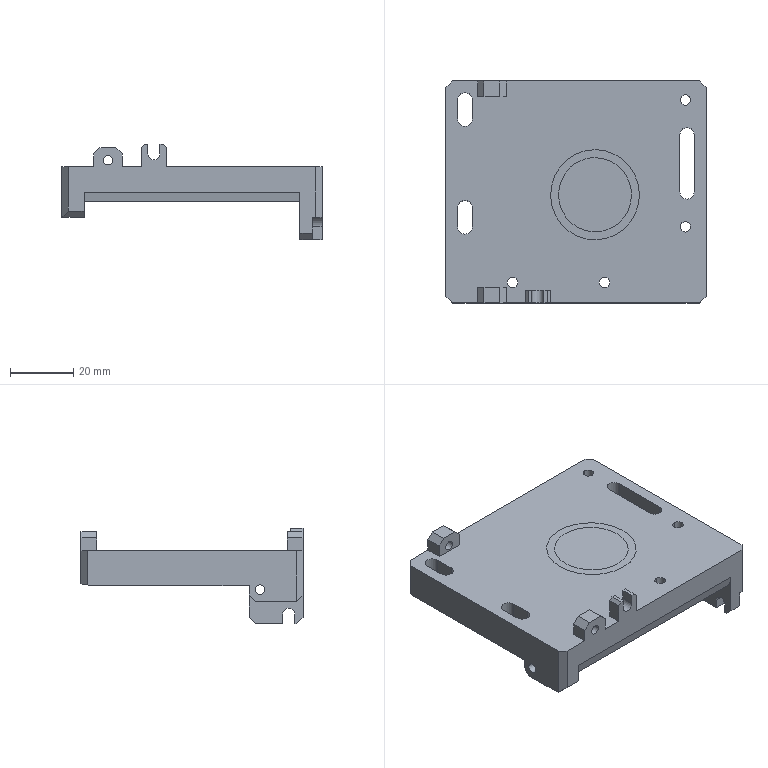NC program | NX | posted with a generic post | part box 82 x 70 x 30 mm
Lines 2119 to 3882 of 5501, first 1664 of 1756 lines:
(CAVITY_MILL_COPY_COPY_1 , TOOL : D4)
N4230 T04 M6
N4232 G54
N4234 G17 G0 G90 X-28.2 Y14.17 B0. C0. S9500 M3
N4236 G43 Z30. H4
N4238 Z1.25
N4240 G94 G1 Z-0.25 F1000.
N4242 X-28.364 Y14.123
N4244 G3 X-29.062 Y13.407 R1.
N4246 G2 X-30.376 Y12. R2. F1100.
N4248 X-29.062 Y10.593 R2.
N4250 G3 X-28.364 Y9.877 R1.
N4252 G1 X-28.2 Y9.83
N4254 Z1.25
N4256 G0 Y14.17 Z1.
N4258 G1 Z-0.5 F1000.
N4260 X-28.364 Y14.123
N4262 G3 X-29.062 Y13.407 R1.
N4264 G2 X-30.376 Y12. R2. F1100.
N4266 X-29.062 Y10.593 R2.
N4268 G3 X-28.364 Y9.877 R1.
N4270 G1 X-28.2 Y9.83
N4272 Z1.
N4274 G0 Y14.17 Z0.75
N4276 G1 Z-0.75 F1000.
N4278 X-28.364 Y14.123
N4280 G3 X-29.062 Y13.407 R1.
N4282 G2 X-30.376 Y12. R2. F1100.
N4284 X-29.062 Y10.593 R2.
N4286 G3 X-28.364 Y9.877 R1.
N4288 G1 X-28.2 Y9.83
N4290 Z0.75
N4292 G0 Y14.17 Z0.5
N4294 G1 Z-1. F1000.
N4296 X-28.364 Y14.123
N4298 G3 X-29.062 Y13.407 R1.
N4300 G2 X-30.376 Y12. R2. F1100.
N4302 X-29.062 Y10.593 R2.
N4304 G3 X-28.364 Y9.877 R1.
N4306 G1 X-28.2 Y9.83
N4308 Z0.5
N4310 G0 X-28.15 Y21.012 Z0.2
N4312 G1 Z-1.3 F1000.
N4314 X-29.294 Y20.491
N4316 G3 X-29.875 Y19.677 R1.
N4318 G1 X-31.666 Y19.85
N4320 X-31.661 Y19.9 F1100.
N4322 X-33.397
N4324 Y19.8
N4326 X-31.671
N4328 X-31.666 Y19.85
N4330 X-29.875 Y19.677
N4332 X-29.872 Y19.706
N4334 G2 X-28.845 Y21.476 R2.52
N4336 G1 X-28.779 Y21.523
N4338 G3 X-28.662 Y22.214 R0.5
N4340 G2 X-30. Y21.7 R2.
N4342 G1 X-35.
N4344 G2 X-36.492 Y22.373 R2.009
N4346 G3 X-36.51 Y21.738 R0.5
N4348 X-35.197 Y21.229 R2.489
N4350 G1 Y18.472
N4352 G3 X-36.491 Y17.982 R2.48
N4354 X-36.48 Y17.346 R0.5
N4356 G2 X-35. Y18. R2.
N4358 G1 X-31.
N4360 G2 X-29.368 Y17.156 R2.
N4362 G3 X-29.319 Y17.841 R0.5
N4364 G2 X-29.875 Y19.677 R2.52
N4366 X-29.294 Y20.491 R1.
N4368 G1 X-28.15 Y21.012
N4370 Z0.2
N4372 G0 X-28.445 Y17.989 Z-0.1
N4374 G1 Z-1.6 F1000.
N4376 X-29.322 Y18.673
N4378 G2 X-29.697 Y19.6 R1.
N4380 X-28.743 Y21.245 R2.52 F1100.
N4382 G3 X-28.642 Y21.931 R0.5
N4384 G2 X-30. Y21.4 R2.
N4386 G1 X-35.
N4388 G2 X-36.608 Y22.214 R2.003
N4390 G3 X-36.685 Y21.582 R0.5
N4392 X-35.197 Y20.928 R2.483
N4394 G1 Y18.472
N4396 G3 X-36.587 Y17.906 R2.48
N4398 X-36.544 Y17.271 R0.5
N4400 G2 X-35. Y18. R2.
N4402 G1 X-31.
N4404 G2 X-29.313 Y17.074 R2.
N4406 G3 X-29.23 Y17.756 R0.5
N4408 G2 X-29.697 Y19.6 R2.52
N4410 X-29.083 Y20.388 R1.
N4412 G1 X-28.053 Y20.806
N4414 Z-0.1
N4416 G0 X-28.354 Y17.868 Z-0.4
N4418 G1 Z-1.9 F1000.
N4420 X-29.2 Y18.616
N4422 G2 X-29.519 Y19.563 R1.
N4424 X-28.68 Y20.985 R2.52 F1100.
N4426 G3 X-28.604 Y21.667 R0.5
N4428 G2 X-30. Y21.1 R2.
N4430 G1 X-35.
N4432 G2 X-36.599 Y21.901 R2.004
N4434 G3 X-36.67 Y21.269 R0.5
N4436 X-35.197 Y20.628 R2.484
N4438 G1 Y18.472
N4440 G3 X-36.662 Y17.841 R2.48
N4442 X-36.594 Y17.208 R0.5
N4444 G2 X-35. Y18. R2.
N4446 G1 X-31.
N4448 G2 X-29.263 Y16.992 R2.
N4450 G3 X-29.147 Y17.668 R0.5
N4452 G2 X-29.519 Y19.563 R2.52
N4454 X-28.857 Y20.313 R1.
N4456 G1 X-27.937 Y20.622
N4458 Z-0.4
N4460 G0 X-28.263 Y17.735 Z-0.7
N4462 G1 Z-2.2 F1000.
N4464 X-29.073 Y18.546
N4466 G2 X-29.33 Y19.513 R1.
N4468 X-28.614 Y20.702 R2.52 F1100.
N4470 G1 X-28.516 Y20.793
N4472 G3 X-28.486 Y21.494 R0.5
N4474 G2 X-30. Y20.8 R2.
N4476 G1 X-35.
N4478 G2 X-36.681 Y21.717 R2.
N4480 G3 X-36.798 Y21.091 R0.5
N4482 X-35.197 Y20.328 R2.48
N4484 G1 Y18.472
N4486 G3 X-36.741 Y17.766 R2.48
N4488 X-36.645 Y17.137 R0.5
N4490 G2 X-35. Y18. R2.
N4492 G1 X-31.
N4494 G2 X-29.215 Y16.901 R2.
N4496 G3 X-29.064 Y17.571 R0.5
N4498 G2 X-29.33 Y19.513 R2.52
N4500 X-28.622 Y20.219 R1.
N4502 G1 X-27.77 Y20.446
N4504 Z-0.7
N4506 G0 X-28.192 Y17.619 Z-1.
N4508 G1 Z-2.5 F1000.
N4510 X-28.966 Y18.482
N4512 G2 X-29.172 Y19.461 R1.
N4514 X-28.537 Y20.481 R2.52 F1100.
N4516 G3 X-28.509 Y21.167 R0.5
N4518 G2 X-30. Y20.5 R2.
N4520 G1 X-35.
N4522 G2 X-36.694 Y21.437 R2.
N4524 G3 X-36.818 Y20.813 R0.5
N4526 X-35.197 Y20.028 R2.48
N4528 G1 Y18.472
N4530 G3 X-36.808 Y17.698 R2.48
N4532 X-36.688 Y17.073 R0.5
N4534 G2 X-35. Y18. R2.
N4536 G1 X-31.
N4538 G2 X-29.177 Y16.823 R2.
N4540 G3 X-28.998 Y17.486 R0.5
N4542 G2 X-29.172 Y19.461 R2.52
N4544 X-28.428 Y20.129 R1.
N4546 G1 X-27.713 Y20.279
N4548 Z-1.
N4550 G0 X-28.121 Y17.491 Z-1.3
N4552 G1 Z-2.8 F1000.
N4554 X-28.855 Y18.407
N4556 G2 X-29.006 Y19.396 R1.
N4558 X-28.466 Y20.235 R2.52 F1100.
N4560 G3 X-28.461 Y20.926 R0.5
N4562 G2 X-30. Y20.2 R2.004
N4564 G1 X-35.
N4566 G2 X-36.73 Y21.199 R2.003
N4568 G3 X-36.876 Y20.58 R0.5
N4570 X-35.197 Y19.728 R2.483
N4572 G1 Y18.472
N4574 G3 X-36.872 Y17.627 R2.48
N4576 X-36.728 Y17.007 R0.5
N4578 G2 X-35. Y18. R2.
N4580 G1 X-31.
N4582 G2 X-29.141 Y16.738 R2.
N4584 G3 X-28.931 Y17.392 R0.5
N4586 G2 X-29.006 Y19.396 R2.52
N4588 X-28.225 Y20.021 R1.
N4590 G1 X-27.613 Y20.114
N4592 Z-1.3
N4594 G0 X-28.078 Y17.405 Z-1.6
N4596 G1 Z-3.1 F1000.
N4598 X-28.783 Y18.356
N4600 G2 X-28.898 Y19.349 R1.
N4602 X-28.435 Y20.059 R2.52 F1100.
N4604 G3 X-28.443 Y20.745 R0.5
N4606 G2 X-30. Y20. R2.
N4608 G1 X-35.
N4610 G2 X-36.753 Y21.037 R2.
N4612 G3 X-36.912 Y20.421 R0.5
N4614 X-35.198 Y19.528 R2.48
N4616 G1 Y18.472
N4618 G3 X-36.912 Y17.579 R2.48
N4620 X-36.753 Y16.963 R0.5
N4622 G2 X-35. Y18. R2.
N4624 G1 X-31.
N4626 G2 X-29.12 Y16.682 R2.
N4628 G3 X-28.89 Y17.329 R0.5
N4630 G2 X-28.898 Y19.349 R2.52
N4632 X-28.095 Y19.945 R1.
N4634 G1 X-27.563 Y20.007
N4636 Z-1.6
N4638 G0 X-28.078 Y17.405 Z-1.9
N4640 G1 Z-3.4 F1000.
N4642 X-28.783 Y18.356
N4644 G2 X-28.898 Y19.349 R1.
N4646 X-28.435 Y20.059 R2.52 F1100.
N4648 G3 X-28.442 Y20.745 R0.5
N4650 G2 X-30. Y20. R2.
N4652 G1 X-35.
N4654 G2 X-36.753 Y21.037 R2.
N4656 G3 X-36.912 Y20.421 R0.5
N4658 X-35.198 Y19.528 R2.48
N4660 G1 Y18.472
N4662 G3 X-36.912 Y17.579 R2.48
N4664 X-36.753 Y16.963 R0.5
N4666 G2 X-35. Y18. R2.
N4668 G1 X-31.
N4670 G2 X-29.12 Y16.682 R2.
N4672 G3 X-28.89 Y17.329 R0.5
N4674 G2 X-28.898 Y19.349 R2.52
N4676 X-28.095 Y19.945 R1.
N4678 G1 X-27.563 Y20.007
N4680 Z-1.9
N4682 G0 X-28.078 Y17.405 Z-2.2
N4684 G1 Z-3.7 F1000.
N4686 X-28.783 Y18.356
N4688 G2 X-28.898 Y19.349 R1.
N4690 X-28.435 Y20.059 R2.52 F1100.
N4692 G3 X-28.442 Y20.745 R0.5
N4694 G2 X-30. Y20. R2.
N4696 G1 X-35.
N4698 G2 X-36.753 Y21.037 R2.
N4700 G3 X-36.912 Y20.421 R0.5
N4702 X-35.198 Y19.528 R2.48
N4704 G1 Y18.472
N4706 G3 X-36.912 Y17.579 R2.48
N4708 X-36.753 Y16.963 R0.5
N4710 G2 X-35. Y18. R2.
N4712 G1 X-31.
N4714 G2 X-29.12 Y16.682 R2.
N4716 G3 X-28.89 Y17.329 R0.5
N4718 G2 X-28.898 Y19.349 R2.52
N4720 X-28.095 Y19.945 R1.
N4722 G1 X-27.563 Y20.007
N4724 Z-2.2
N4726 G0 X-28.078 Y17.405 Z-2.5
N4728 G1 Z-4. F1000.
N4730 X-28.783 Y18.356
N4732 G2 X-28.898 Y19.349 R1.
N4734 X-28.435 Y20.059 R2.52 F1100.
N4736 G3 X-28.443 Y20.745 R0.5
N4738 G2 X-30. Y20. R2.
N4740 G1 X-35.
N4742 G2 X-36.753 Y21.037 R2.
N4744 G3 X-36.912 Y20.421 R0.5
N4746 X-35.198 Y19.528 R2.48
N4748 G1 Y18.472
N4750 G3 X-36.912 Y17.579 R2.48
N4752 X-36.753 Y16.963 R0.5
N4754 G2 X-35. Y18. R2.
N4756 G1 X-31.
N4758 G2 X-29.12 Y16.682 R2.
N4760 G3 X-28.89 Y17.329 R0.5
N4762 G2 X-28.898 Y19.349 R2.52
N4764 X-28.095 Y19.945 R1.
N4766 G1 X-27.563 Y20.007
N4768 Z-2.5
N4770 G0 X-28.078 Y17.405 Z-2.8
N4772 G1 Z-4.3 F1000.
N4774 X-28.783 Y18.356
N4776 G2 X-28.898 Y19.349 R1.
N4778 X-28.435 Y20.059 R2.52 F1100.
N4780 G3 X-28.443 Y20.745 R0.5
N4782 G2 X-30. Y20. R2.
N4784 G1 X-35.
N4786 G2 X-36.753 Y21.037 R2.
N4788 G3 X-36.912 Y20.421 R0.5
N4790 X-35.198 Y19.528 R2.48
N4792 G1 Y18.472
N4794 G3 X-36.912 Y17.579 R2.48
N4796 X-36.753 Y16.963 R0.5
N4798 G2 X-35. Y18. R2.
N4800 G1 X-31.
N4802 G2 X-29.12 Y16.682 R2.
N4804 G3 X-28.89 Y17.329 R0.5
N4806 G2 X-28.898 Y19.349 R2.52
N4808 X-28.095 Y19.945 R1.
N4810 G1 X-27.563 Y20.007
N4812 Z-2.8
N4814 G0 X-28.078 Y17.405 Z-3.1
N4816 G1 Z-4.6 F1000.
N4818 X-28.783 Y18.356
N4820 G2 X-28.898 Y19.349 R1.
N4822 X-28.435 Y20.059 R2.52 F1100.
N4824 G3 X-28.443 Y20.745 R0.5
N4826 G2 X-30. Y20. R2.
N4828 G1 X-35.
N4830 G2 X-36.753 Y21.037 R2.
N4832 G3 X-36.912 Y20.421 R0.5
N4834 X-35.198 Y19.528 R2.48
N4836 G1 Y18.472
N4838 G3 X-36.912 Y17.579 R2.48
N4840 X-36.753 Y16.963 R0.5
N4842 G2 X-35. Y18. R2.
N4844 G1 X-31.
N4846 G2 X-29.12 Y16.682 R2.
N4848 G3 X-28.89 Y17.329 R0.5
N4850 G2 X-28.898 Y19.349 R2.52
N4852 X-28.095 Y19.945 R1.
N4854 G1 X-27.563 Y20.007
N4856 Z-3.1
N4858 G0 X-28.078 Y17.405 Z-3.4
N4860 G1 Z-4.9 F1000.
N4862 X-28.783 Y18.356
N4864 G2 X-28.898 Y19.349 R1.
N4866 X-28.435 Y20.059 R2.52 F1100.
N4868 G3 X-28.443 Y20.745 R0.5
N4870 G2 X-30. Y20. R2.
N4872 G1 X-35.
N4874 G2 X-36.753 Y21.037 R2.
N4876 G3 X-36.912 Y20.421 R0.5
N4878 X-35.198 Y19.528 R2.48
N4880 G1 Y18.472
N4882 G3 X-36.912 Y17.579 R2.48
N4884 X-36.753 Y16.963 R0.5
N4886 G2 X-35. Y18. R2.
N4888 G1 X-31.
N4890 G2 X-29.12 Y16.682 R2.
N4892 G3 X-28.89 Y17.329 R0.5
N4894 G2 X-28.898 Y19.349 R2.52
N4896 X-28.095 Y19.945 R1.
N4898 G1 X-27.563 Y20.007
N4900 Z-3.4
N4902 G0 X-28.078 Y17.405 Z-3.7
N4904 G1 Z-5.2 F1000.
N4906 X-28.783 Y18.356
N4908 G2 X-28.898 Y19.349 R1.
N4910 X-28.435 Y20.059 R2.52 F1100.
N4912 G3 X-28.443 Y20.745 R0.5
N4914 G2 X-30. Y20. R2.
N4916 G1 X-35.
N4918 G2 X-36.753 Y21.037 R2.
N4920 G3 X-36.912 Y20.421 R0.5
N4922 X-35.198 Y19.528 R2.48
N4924 G1 Y18.472
N4926 G3 X-36.912 Y17.579 R2.48
N4928 X-36.753 Y16.963 R0.5
N4930 G2 X-35. Y18. R2.
N4932 G1 X-31.
N4934 G2 X-29.12 Y16.682 R2.
N4936 G3 X-28.89 Y17.329 R0.5
N4938 G2 X-28.898 Y19.349 R2.52
N4940 X-28.095 Y19.945 R1.
N4942 G1 X-27.563 Y20.007
N4944 Z-3.7
N4946 G0 X-28.078 Y17.405 Z-4.
N4948 G1 Z-5.5 F1000.
N4950 X-28.783 Y18.356
N4952 G2 X-28.898 Y19.349 R1.
N4954 X-28.435 Y20.059 R2.52 F1100.
N4956 G3 X-28.443 Y20.745 R0.5
N4958 G2 X-30. Y20. R2.
N4960 G1 X-35.
N4962 G2 X-36.753 Y21.037 R2.
N4964 G3 X-36.912 Y20.421 R0.5
N4966 X-35.198 Y19.528 R2.48
N4968 G1 Y18.472
N4970 G3 X-36.912 Y17.579 R2.48
N4972 X-36.753 Y16.963 R0.5
N4974 G2 X-35. Y18. R2.
N4976 G1 X-31.
N4978 G2 X-29.12 Y16.682 R2.
N4980 G3 X-28.89 Y17.329 R0.5
N4982 G2 X-28.898 Y19.349 R2.52
N4984 X-28.095 Y19.945 R1.
N4986 G1 X-27.563 Y20.007
N4988 Z-4.
N4990 G0 X-28.078 Y17.405 Z-4.3
N4992 G1 Z-5.8 F1000.
N4994 X-28.783 Y18.356
N4996 G2 X-28.898 Y19.349 R1.
N4998 X-28.435 Y20.059 R2.52 F1100.
N5000 G3 X-28.443 Y20.745 R0.5
N5002 G2 X-30. Y20. R2.
N5004 G1 X-35.
N5006 G2 X-36.753 Y21.037 R2.
N5008 G3 X-36.912 Y20.421 R0.5
N5010 X-35.198 Y19.528 R2.48
N5012 G1 Y18.472
N5014 G3 X-36.912 Y17.579 R2.48
N5016 X-36.753 Y16.963 R0.5
N5018 G2 X-35. Y18. R2.
N5020 G1 X-31.
N5022 G2 X-29.12 Y16.682 R2.
N5024 G3 X-28.89 Y17.329 R0.5
N5026 G2 X-28.898 Y19.349 R2.52
N5028 X-28.095 Y19.945 R1.
N5030 G1 X-27.563 Y20.007
N5032 Z-4.3
N5034 G0 X-28.078 Y17.405 Z-4.6
N5036 G1 Z-6.1 F1000.
N5038 X-28.783 Y18.356
N5040 G2 X-28.898 Y19.349 R1.
N5042 X-28.435 Y20.059 R2.52 F1100.
N5044 G3 X-28.443 Y20.745 R0.5
N5046 G2 X-30. Y20. R2.
N5048 G1 X-35.
N5050 G2 X-36.753 Y21.037 R2.
N5052 G3 X-36.912 Y20.421 R0.5
N5054 X-35.198 Y19.528 R2.48
N5056 G1 Y18.472
N5058 G3 X-36.912 Y17.579 R2.48
N5060 X-36.753 Y16.963 R0.5
N5062 G2 X-35. Y18. R2.
N5064 G1 X-31.
N5066 G2 X-29.12 Y16.682 R2.
N5068 G3 X-28.89 Y17.329 R0.5
N5070 G2 X-28.898 Y19.349 R2.52
N5072 X-28.095 Y19.945 R1.
N5074 G1 X-27.563 Y20.007
N5076 Z-4.6
N5078 G0 X-28.078 Y17.405 Z-4.9
N5080 G1 Z-6.4 F1000.
N5082 X-28.783 Y18.356
N5084 G2 X-28.898 Y19.349 R1.
N5086 X-28.435 Y20.059 R2.52 F1100.
N5088 G3 X-28.443 Y20.745 R0.5
N5090 G2 X-30. Y20. R2.
N5092 G1 X-35.
N5094 G2 X-36.753 Y21.037 R2.
N5096 G3 X-36.912 Y20.421 R0.5
N5098 X-35.198 Y19.528 R2.48
N5100 G1 Y18.472
N5102 G3 X-36.912 Y17.579 R2.48
N5104 X-36.753 Y16.963 R0.5
N5106 G2 X-35. Y18. R2.
N5108 G1 X-31.
N5110 G2 X-29.12 Y16.682 R2.
N5112 G3 X-28.89 Y17.329 R0.5
N5114 G2 X-28.898 Y19.349 R2.52
N5116 X-28.095 Y19.945 R1.
N5118 G1 X-27.563 Y20.007
N5120 Z-4.9
N5122 G0 X-28.078 Y17.405 Z-5.2
N5124 G1 Z-6.7 F1000.
N5126 X-28.783 Y18.356
N5128 G2 X-28.898 Y19.349 R1.
N5130 X-28.435 Y20.059 R2.52 F1100.
N5132 G3 X-28.443 Y20.745 R0.5
N5134 G2 X-30. Y20. R2.
N5136 G1 X-35.
N5138 G2 X-36.753 Y21.037 R2.
N5140 G3 X-36.912 Y20.421 R0.5
N5142 X-35.198 Y19.528 R2.48
N5144 G1 Y18.472
N5146 G3 X-36.912 Y17.579 R2.48
N5148 X-36.753 Y16.963 R0.5
N5150 G2 X-35. Y18. R2.
N5152 G1 X-31.
N5154 G2 X-29.12 Y16.682 R2.
N5156 G3 X-28.89 Y17.329 R0.5
N5158 G2 X-28.898 Y19.349 R2.52
N5160 X-28.095 Y19.945 R1.
N5162 G1 X-27.563 Y20.007
N5164 Z-5.2
N5166 G0 X-28.078 Y17.405 Z-5.5
N5168 G1 Z-7. F1000.
N5170 X-28.783 Y18.356
N5172 G2 X-28.898 Y19.349 R1.
N5174 X-28.435 Y20.059 R2.52 F1100.
N5176 G3 X-28.443 Y20.745 R0.5
N5178 G2 X-30. Y20. R2.
N5180 G1 X-35.
N5182 G2 X-36.753 Y21.037 R2.
N5184 G3 X-36.912 Y20.421 R0.5
N5186 X-35.198 Y19.528 R2.48
N5188 G1 Y18.472
N5190 G3 X-36.912 Y17.579 R2.48
N5192 X-36.753 Y16.963 R0.5
N5194 G2 X-35. Y18. R2.
N5196 G1 X-31.
N5198 G2 X-29.12 Y16.682 R2.
N5200 G3 X-28.89 Y17.329 R0.5
N5202 G2 X-28.898 Y19.349 R2.52
N5204 X-28.095 Y19.945 R1.
N5206 G1 X-27.563 Y20.007
N5208 Z-5.5
N5210 G0 Z30.
N5212 X-28.2 Y14.17
N5214 Z0.2
N5216 G1 Z-1.3 F1000.
N5218 X-28.364 Y14.123
N5220 G3 X-29.062 Y13.407 R1.
N5222 G2 X-30.376 Y12. R2. F1100.
N5224 X-29.062 Y10.593 R2.
N5226 G3 X-28.364 Y9.877 R1.
N5228 G1 X-28.2 Y9.83
N5230 Z0.2
N5232 G0 Y14.17 Z-0.1
N5234 G1 Z-1.6 F1000.
N5236 X-28.364 Y14.123
N5238 G3 X-29.062 Y13.407 R1.
N5240 G2 X-30.376 Y12. R2. F1100.
N5242 X-29.062 Y10.593 R2.
N5244 G3 X-28.364 Y9.877 R1.
N5246 G1 X-28.2 Y9.83
N5248 Z-0.1
N5250 G0 Y14.17 Z-0.4
N5252 G1 Z-1.9 F1000.
N5254 X-28.364 Y14.123
N5256 G3 X-29.062 Y13.407 R1.
N5258 G2 X-30.376 Y12. R2. F1100.
N5260 X-29.062 Y10.593 R2.
N5262 G3 X-28.364 Y9.877 R1.
N5264 G1 X-28.2 Y9.83
N5266 Z-0.4
N5268 G0 Y14.17 Z-0.7
N5270 G1 Z-2.2 F1000.
N5272 X-28.364 Y14.123
N5274 G3 X-29.062 Y13.407 R1.
N5276 G2 X-30.376 Y12. R2. F1100.
N5278 X-29.062 Y10.593 R2.
N5280 G3 X-28.364 Y9.877 R1.
N5282 G1 X-28.2 Y9.83
N5284 Z-0.7
N5286 G0 Y14.17 Z-1.
N5288 G1 Z-2.5 F1000.
N5290 X-28.364 Y14.123
N5292 G3 X-29.062 Y13.407 R1.
N5294 G2 X-30.376 Y12. R2. F1100.
N5296 X-29.062 Y10.593 R2.
N5298 G3 X-28.364 Y9.877 R1.
N5300 G1 X-28.2 Y9.83
N5302 Z-1.
N5304 G0 Y14.17 Z-1.3
N5306 G1 Z-2.8 F1000.
N5308 X-28.364 Y14.123
N5310 G3 X-29.062 Y13.407 R1.
N5312 G2 X-30.376 Y12. R2. F1100.
N5314 X-29.062 Y10.593 R2.
N5316 G3 X-28.364 Y9.877 R1.
N5318 G1 X-28.2 Y9.83
N5320 Z-1.3
N5322 G0 Y14.17 Z-1.6
N5324 G1 Z-3.1 F1000.
N5326 X-28.364 Y14.123
N5328 G3 X-29.062 Y13.407 R1.
N5330 G2 X-29.372 Y12.738 R2. F1100.
N5332 X-30.355 Y12. R1.958
N5334 X-29.375 Y11.265 R1.952
N5336 X-29.062 Y10.593 R2.
N5338 G3 X-28.364 Y9.877 R1.
N5340 G1 X-28.2 Y9.83
N5342 Z-1.6
N5344 G0 Y14.156 Z-1.9
N5346 G1 Z-3.4 F1000.
N5348 X-28.366 Y14.107
N5350 G3 X-29.053 Y13.381 R1.
N5352 G2 X-30.252 Y12. R1.977 F1100.
N5354 X-29.052 Y10.612 R1.979
N5356 G3 X-28.367 Y9.884 R1.
N5358 G1 X-28.2 Y9.833
N5360 Z-1.9
N5362 G0 Y14.124 Z-2.2
N5364 G1 Z-3.7 F1000.
N5366 X-28.373 Y14.069
N5368 G3 X-29.045 Y13.329 R1.
N5370 G2 X-30.05 Y12.001 R1.981 F1100.
N5372 X-29.049 Y10.685 R1.988
N5374 G3 X-28.37 Y9.95 R1.
N5376 G1 X-28.2 Y9.897
N5378 Z-2.2
N5380 G0 Y14.094 Z-2.5
N5382 G1 Z-4. F1000.
N5384 X-28.388 Y14.025
N5386 G3 X-29.031 Y13.26 R1.
N5388 G2 X-29.805 Y11.996 R2.023 F1100.
N5390 X-29.034 Y10.765 R1.987
N5392 G3 X-28.383 Y10.006 R1.
N5394 G1 X-28.2 Y9.941
N5396 Z-2.5
N5398 G0 Y13.998 Z-2.8
N5400 G1 Z-4.3 F1000.
N5402 X-28.409 Y13.911
N5404 G3 X-29.016 Y13.116 R1.
N5406 G2 X-29.552 Y12.002 R1.969 F1100.
N5408 X-29.018 Y10.89 R1.99
N5410 G3 X-28.407 Y10.098 R1.
N5412 G1 X-28.2 Y10.012
N5414 Z-2.8
N5416 G0 Y13.908 Z-3.1
N5418 G1 Z-4.6 F1000.
N5420 X-28.462 Y13.772
N5422 G3 X-29.002 Y12.93 R1.
N5424 G2 X-29.272 Y12.002 R2.068 F1100.
N5426 X-29.001 Y11.043 R2.095
N5428 G3 X-28.471 Y10.195 R1.
N5430 G1 X-28.2 Y10.051
N5432 Z-3.1
N5434 G0 Z30.
N5436 X-37.8 Y9.83
N5438 Z1.25
N5440 G1 Z-0.25 F1000.
N5442 X-37.636 Y9.877
N5444 G3 X-36.938 Y10.593 R1.
N5446 G2 X-35.625 Y12. R2. F1100.
N5448 X-36.938 Y13.407 R2.
N5450 G3 X-37.636 Y14.123 R1.
N5452 G1 X-37.8 Y14.17
N5454 Z1.25
N5456 G0 Y9.83 Z1.
N5458 G1 Z-0.5 F1000.
N5460 X-37.636 Y9.877
N5462 G3 X-36.938 Y10.593 R1.
N5464 G2 X-35.625 Y12. R2. F1100.
N5466 X-36.938 Y13.407 R2.
N5468 G3 X-37.636 Y14.123 R1.
N5470 G1 X-37.8 Y14.17
N5472 Z1.
N5474 G0 Y9.83 Z0.75
N5476 G1 Z-0.75 F1000.
N5478 X-37.636 Y9.877
N5480 G3 X-36.938 Y10.593 R1.
N5482 G2 X-35.625 Y12. R2. F1100.
N5484 X-36.938 Y13.407 R2.
N5486 G3 X-37.636 Y14.123 R1.
N5488 G1 X-37.8 Y14.17
N5490 Z0.75
N5492 G0 Y9.83 Z0.5
N5494 G1 Z-1. F1000.
N5496 X-37.636 Y9.877
N5498 G3 X-36.938 Y10.593 R1.
N5500 G2 X-35.625 Y12. R2. F1100.
N5502 X-36.938 Y13.407 R2.
N5504 G3 X-37.636 Y14.123 R1.
N5506 G1 X-37.8 Y14.17
N5508 Z0.5
N5510 G0 Y9.83 Z0.2
N5512 G1 Z-1.3 F1000.
N5514 X-37.636 Y9.877
N5516 G3 X-36.938 Y10.593 R1.
N5518 G2 X-35.625 Y12. R2. F1100.
N5520 X-36.938 Y13.407 R2.
N5522 G3 X-37.636 Y14.123 R1.
N5524 G1 X-37.8 Y14.17
N5526 Z0.2
N5528 G0 Y9.83 Z-0.1
N5530 G1 Z-1.6 F1000.
N5532 X-37.636 Y9.877
N5534 G3 X-36.938 Y10.593 R1.
N5536 G2 X-35.625 Y12. R2. F1100.
N5538 X-36.938 Y13.407 R2.
N5540 G3 X-37.636 Y14.123 R1.
N5542 G1 X-37.8 Y14.17
N5544 Z-0.1
N5546 G0 Y9.83 Z-0.4
N5548 G1 Z-1.9 F1000.
N5550 X-37.636 Y9.877
N5552 G3 X-36.938 Y10.593 R1.
N5554 G2 X-35.625 Y12. R2. F1100.
N5556 X-36.938 Y13.407 R2.
N5558 G3 X-37.636 Y14.123 R1.
N5560 G1 X-37.8 Y14.17
N5562 Z-0.4
N5564 G0 Y9.83 Z-0.7
N5566 G1 Z-2.2 F1000.
N5568 X-37.636 Y9.877
N5570 G3 X-36.938 Y10.593 R1.
N5572 G2 X-35.625 Y12. R2. F1100.
N5574 X-36.938 Y13.407 R2.
N5576 G3 X-37.636 Y14.123 R1.
N5578 G1 X-37.8 Y14.17
N5580 Z-0.7
N5582 G0 Y9.83 Z-1.
N5584 G1 Z-2.5 F1000.
N5586 X-37.636 Y9.877
N5588 G3 X-36.938 Y10.593 R1.
N5590 G2 X-35.625 Y12. R2. F1100.
N5592 X-36.938 Y13.407 R2.
N5594 G3 X-37.636 Y14.123 R1.
N5596 G1 X-37.8 Y14.17
N5598 Z-1.
N5600 G0 Y9.83 Z-1.3
N5602 G1 Z-2.8 F1000.
N5604 X-37.636 Y9.877
N5606 G3 X-36.938 Y10.593 R1.
N5608 G2 X-35.625 Y12. R2. F1100.
N5610 X-36.938 Y13.407 R2.
N5612 G3 X-37.636 Y14.123 R1.
N5614 G1 X-37.8 Y14.17
N5616 Z-1.3
N5618 G0 Y9.83 Z-1.6
N5620 G1 Z-3.1 F1000.
N5622 X-37.636 Y9.877
N5624 G3 X-36.938 Y10.593 R1.
N5626 G2 X-36.62 Y11.273 R2. F1100.
N5628 X-35.641 Y12. R1.936
N5630 X-36.715 Y12.871 R1.953
N5632 X-36.938 Y13.407 R2.
N5634 G3 X-37.636 Y14.123 R1.
N5636 G1 X-37.8 Y14.17
N5638 Z-1.6
N5640 G0 Y9.822 Z-1.9
N5642 G1 Z-3.4 F1000.
N5644 X-37.632 Y9.874
N5646 G3 X-36.95 Y10.605 R1.
N5648 G2 X-35.757 Y11.997 R1.981 F1100.
N5650 X-36.153 Y12.219 R3.507
N5652 X-36.604 Y12.647 R2.331
N5654 X-36.774 Y12.922 R2.63
N5656 X-36.953 Y13.401 R1.909
N5658 G3 X-37.632 Y14.135 R1.
N5660 G1 X-37.8 Y14.187
N5662 Z-1.9
N5664 G0 Y9.871 Z-2.2
N5666 G1 Z-3.7 F1000.
N5668 X-37.627 Y9.926
N5670 G3 X-36.954 Y10.666 R1.
N5672 G2 X-36.153 Y11.876 R2.005 F1100.
N5674 G1 X-35.994 Y11.984
N5676 X-35.959 Y11.997
N5678 G2 X-36.894 Y13.112 R2.069
N5680 X-36.954 Y13.324 R1.922
N5682 G3 X-37.63 Y14.061 R1.
N5684 G1 X-37.8 Y14.114
N5686 Z-2.2
N5688 G0 Y9.931 Z-2.5
N5690 G1 Z-4. F1000.
N5692 X-37.616 Y9.996
N5694 G3 X-36.967 Y10.757 R1.
N5696 G2 X-36.196 Y11.998 R2.003 F1100.
N5698 X-36.964 Y13.235 R2.022
N5700 G3 X-37.617 Y13.993 R1.
N5702 G1 X-37.8 Y14.056
N5704 Z-2.5
N5706 G0 Y10.025 Z-2.8
N5708 G1 Z-4.3 F1000.
N5710 X-37.595 Y10.108
N5712 G3 X-36.981 Y10.896 R1.
N5714 G2 X-36.452 Y11.998 R2.008 F1100.
N5716 X-36.98 Y13.099 R2.023
N5718 G3 X-37.596 Y13.887 R1.
N5720 G1 X-37.8 Y13.969
N5722 Z-2.8
N5724 G0 Y10.11 Z-3.1
N5726 G1 Z-4.6 F1000.
N5728 X-37.544 Y10.24
N5730 G3 X-36.997 Y11.078 R1.
N5732 G2 X-36.729 Y11.984 R2.046 F1100.
N5734 X-36.998 Y12.946 R2.256
N5736 G3 X-37.54 Y13.786 R1.
N5738 G1 X-37.8 Y13.919
N5740 Z-3.1
N5742 G0 Z30.
(FLOOR_WALL_1_COPY , TOOL : D4)
N5744 X38.187 Y31.917
N5746 Z0.5
N5748 G1 Z-1. F1250.
N5750 X37.2 Y31.346
N5752 G3 X37. Y31. R0.4
N5754 G1 Y22.
N5756 X35.2
N5758 Y31.
N5760 X33.4
N5762 Y22.
N5764 X31.6
N5766 Y31.
N5768 G2 X31.8 Y31.346 R0.4
N5770 G1 X33.798 Y32.5
N5772 Z0.5
N5774 G0 Z30.
N5776 X38.187 Y40.745
N5778 Z-5.5
N5780 G1 Z-7.
N5782 X37.2 Y40.175
N5784 G3 X37. Y39.828 R0.4
N5786 G1 Y33.2
N5788 X35.044
N5790 Y41.784
N5792 X33.828 Y43.
N5794 X33.089
N5796 Y33.2
N5798 X31.133
N5800 Y43.
N5802 X29.178
N5804 Y33.2
N5806 G3 X29.524 Y33.4 R0.4
N5808 G1 Z-5.5
N5810 G0 Z30.
N5812 X38.5 Y19.454
N5814 Z-5.5
N5816 G1 Z-7.
N5818 X36.8
N5820 G3 X37. Y19.8 R0.4
N5822 G1 Y-39.828
N5824 X35.044 Y-41.784
N5826 Y19.8
N5828 X33.089
N5830 Y-43.
N5832 X31.133
N5834 Y19.8
N5836 X29.178
N5838 Y-43.
N5840 X27.222
N5842 Y43.
N5844 X25.267
N5846 Y-43.
N5848 X23.311
N5850 Y43.
N5852 X21.356
N5854 Y-43.
N5856 X19.4
N5858 Y43.
N5860 X17.444
N5862 Y-43.
N5864 X15.489
N5866 Y43.
N5868 X13.533
N5870 Y-43.
N5872 X11.578
N5874 Y43.
N5876 X9.622
N5878 Y-43.
N5880 X7.667
N5882 Y43.
N5884 X5.711
N5886 Y-43.
N5888 X3.756
N5890 Y43.
N5892 X1.8
N5894 Y-43.
N5896 X-0.156
N5898 Y43.
N5900 X-2.111
N5902 Y-43.
N5904 X-4.067
N5906 Y43.
N5908 X-6.022
N5910 Y-43.
N5912 X-7.978
N5914 Y43.
N5916 X-9.933
N5918 Y-43.
N5920 X-11.889
N5922 Y43.
N5924 X-13.844
N5926 Y-43.
N5928 X-15.8
N5930 Y43.
N5932 X-17.756
N5934 Y-43.
N5936 X-19.711
N5938 Y43.
N5940 X-21.667
N5942 Y-43.
N5944 X-23.622
N5946 Y43.
N5948 X-25.578
N5950 Y-43.
N5952 X-27.533
N5954 Y43.
N5956 X-29.489
N5958 Y33.2
N5960 X-31.444
N5962 Y43.
N5964 X-33.4
N5966 Y33.2
N5968 X-35.356
N5970 Y41.473
N5972 G2 X-35.156 Y41.819 R0.4
N5974 G1 X-36.143 Y42.807
N5976 Z-5.5
N5978 G0 Z3.1
N5980 G1 X-29.489 Y33.2 F8000.
N5982 G0 Z-5.5
N5984 G1 Z-7. F1250.
N5986 X-28.
N5988 G2 X-27.8 Y33. R0.2
N5990 G1 Y20.
N5992 G2 X-28. Y19.8 R0.2
N5994 G1 X-29.489
N5996 Y18.2
N5998 X-31.444
N6000 Y19.8
N6002 X-33.4
N6004 Y18.2
N6006 X-35.356
N6008 Y19.8
N6010 Z-5.5
N6012 G0 Z3.1
N6014 G1 X-29.489 Y18.2 F8000.
N6016 G0 Z-5.5
N6018 G1 Z-7. F1250.
N6020 X-29.
N6022 G2 X-28.8 Y18. R0.2
N6024 G1 Y5.99
N6026 G2 X-29. Y5.8 R0.2
N6028 G1 X-29.489
N6030 Y-43.
N6032 X-31.444
N6034 Y5.8
N6036 X-33.4
N6038 Y-43.
N6040 X-33.828
N6042 X-35.356 Y-41.473
N6044 Y5.8
N6046 Z-5.5
N6048 G0 Z30.
N6050 X-38.5 Y20.198
N6052 Z-5.5
N6054 G1 Z-7.
N6056 X-37.346 Y18.2
N6058 G3 X-37. Y18. R0.4
N6060 G1 X-29.
N6062 Y6.
N6064 X-37.
N6066 G3 X-37.346 Y5.8 R0.4
N6068 G1 X-38.5 Y3.802
N6070 Z-5.5
N6072 G0 Z3.1
N6074 G1 X38.5 Y17.802 F8000.
N6076 G0 Z-5.5
N6078 G1 Z-7. F1250.
N6080 X37.346 Y19.8
N6082 G3 X37. Y20. R0.4
N6084 G1 X28.
N6086 Y33.
N6088 X37.
N6090 G3 X37.346 Y33.2 R0.4
N6092 G1 X38.5 Y35.198
N6094 Z-5.5
N6096 G0 Z3.1
N6098 G1 X-38.5 F8000.
N6100 G0 Z-5.5
N6102 G1 Z-7. F1250.
N6104 X-37.346 Y33.2
N6106 G3 X-37. Y33. R0.4
N6108 G1 X-28.
N6110 Y20.
N6112 X-37.
N6114 G3 X-37.346 Y19.8 R0.4
N6116 G1 X-38.5 Y17.802
N6118 Z-5.5
N6120 G0 Z30.
N6122 X-26.813 Y31.917
N6124 Z0.5
N6126 G1 Z-1.
N6128 X-27.8 Y31.346
N6130 G3 X-28. Y31. R0.4
N6132 G1 Y22.
N6134 X-29.8
N6136 Y31.
N6138 X-31.6
N6140 Y22.
N6142 X-33.4
N6144 Y31.
N6146 G2 X-33.2 Y31.346 R0.4
N6148 G1 X-31.202 Y32.5
N6150 Z0.5
N6152 G0 Z30.
N6154 M5
(CAVITY_MILL_COPY_COPY_2 , TOOL : D3)
N6156 T03 M6
N6158 G54
N6160 G17 G0 G90 X-36.448 Y12.379 B0. C0. S9500 M3
N6162 G43 Z30. H3
N6164 Z1.3
N6166 G94 G1 Z-0.2 F1000.
N6168 X-36.043 Y12.685
N6170 G2 X-35.826 Y11.709 R1.
N6172 G3 X-35.809 Y11.363 R0.5 F1100.
N6174 G2 X-35. Y11.6 R1.5
N6176 G1 X-31.
N6178 G2 X-30.191 Y11.363 R1.5
N6180 G3 X-30.386 Y11.983 R0.5
N6182 G1 X-30.404 Y11.99
N6184 Y12.01
N6186 X-30.386 Y12.017
N6188 G3 X-30.191 Y12.637 R0.5
N6190 G2 X-31. Y12.4 R1.5
N6192 G1 X-35.
N6194 G2 X-35.809 Y12.637 R1.5
N6196 G3 X-35.614 Y12.017 R0.5
N6198 G1 X-35.596 Y12.01
N6200 Y11.99
N6202 X-35.614 Y11.983
N6204 G3 X-35.826 Y11.709 R0.5
N6206 G2 X-36.563 Y11.033 R1.
N6208 G1 X-36.918 Y10.955
N6210 Z1.3
N6212 G0 X-36.448 Y12.379 Z1.1
N6214 G1 Z-0.4 F1000.
N6216 X-36.043 Y12.685
N6218 G2 X-35.826 Y11.709 R1.
N6220 G3 X-35.809 Y11.363 R0.5 F1100.
N6222 G2 X-35. Y11.6 R1.5
N6224 G1 X-31.
N6226 G2 X-30.191 Y11.363 R1.5
N6228 G3 X-30.386 Y11.983 R0.5
N6230 G1 X-30.404 Y11.99
N6232 Y12.01
N6234 X-30.386 Y12.017
N6236 G3 X-30.191 Y12.637 R0.5
N6238 G2 X-31. Y12.4 R1.5
N6240 G1 X-35.
N6242 G2 X-35.809 Y12.637 R1.5
N6244 G3 X-35.614 Y12.017 R0.5
N6246 G1 X-35.596 Y12.01
N6248 Y11.99
N6250 X-35.614 Y11.983
N6252 G3 X-35.826 Y11.709 R0.5
N6254 G2 X-36.563 Y11.033 R1.
N6256 G1 X-36.918 Y10.955
N6258 Z1.1
N6260 G0 X-36.448 Y12.379 Z0.9
N6262 G1 Z-0.6 F1000.
N6264 X-36.043 Y12.685
N6266 G2 X-35.826 Y11.709 R1.
N6268 G3 X-35.809 Y11.363 R0.5 F1100.
N6270 G2 X-35. Y11.6 R1.5
N6272 G1 X-31.
N6274 G2 X-30.191 Y11.363 R1.5
N6276 G3 X-30.386 Y11.983 R0.5
N6278 G1 X-30.404 Y11.99
N6280 Y12.01
N6282 X-30.386 Y12.017
N6284 G3 X-30.191 Y12.637 R0.5
N6286 G2 X-31. Y12.4 R1.5
N6288 G1 X-35.
N6290 G2 X-35.809 Y12.637 R1.5
N6292 G3 X-35.614 Y12.017 R0.5
N6294 G1 X-35.596 Y12.01
N6296 Y11.99
N6298 X-35.614 Y11.983
N6300 G3 X-35.826 Y11.709 R0.5
N6302 G2 X-36.563 Y11.033 R1.
N6304 G1 X-36.918 Y10.955
N6306 Z0.9
N6308 G0 X-36.448 Y12.379 Z0.7
N6310 G1 Z-0.8 F1000.
N6312 X-36.043 Y12.685
N6314 G2 X-35.826 Y11.709 R1.
N6316 G3 X-35.809 Y11.363 R0.5 F1100.
N6318 G2 X-35. Y11.6 R1.5
N6320 G1 X-31.
N6322 G2 X-30.191 Y11.363 R1.5
N6324 G3 X-30.386 Y11.983 R0.5
N6326 G1 X-30.404 Y11.99
N6328 Y12.01
N6330 X-30.386 Y12.017
N6332 G3 X-30.191 Y12.637 R0.5
N6334 G2 X-31. Y12.4 R1.5
N6336 G1 X-35.
N6338 G2 X-35.809 Y12.637 R1.5
N6340 G3 X-35.614 Y12.017 R0.5
N6342 G1 X-35.596 Y12.01
N6344 Y11.99
N6346 X-35.614 Y11.983
N6348 G3 X-35.826 Y11.709 R0.5
N6350 G2 X-36.563 Y11.033 R1.
N6352 G1 X-36.918 Y10.955
N6354 Z0.7
N6356 G0 X-36.448 Y12.379 Z0.5
N6358 G1 Z-1. F1000.
N6360 X-36.043 Y12.685
N6362 G2 X-35.826 Y11.709 R1.
N6364 G3 X-35.809 Y11.363 R0.5 F1100.
N6366 G2 X-35. Y11.6 R1.5
N6368 G1 X-31.
N6370 G2 X-30.191 Y11.363 R1.5
N6372 G3 X-30.386 Y11.983 R0.5
N6374 G1 X-30.404 Y11.99
N6376 Y12.01
N6378 X-30.386 Y12.017
N6380 G3 X-30.191 Y12.637 R0.5
N6382 G2 X-31. Y12.4 R1.5
N6384 G1 X-35.
N6386 G2 X-35.809 Y12.637 R1.5
N6388 G3 X-35.614 Y12.017 R0.5
N6390 G1 X-35.596 Y12.01
N6392 Y11.99
N6394 X-35.614 Y11.983
N6396 G3 X-35.826 Y11.709 R0.5
N6398 G2 X-36.563 Y11.033 R1.
N6400 G1 X-36.918 Y10.955
N6402 Z0.5
N6404 G0 X-36.448 Y12.379 Z0.3
N6406 G1 Z-1.2 F1000.
N6408 X-36.043 Y12.685
N6410 G2 X-35.826 Y11.709 R1.
N6412 G3 X-35.809 Y11.363 R0.5 F1100.
N6414 G2 X-35. Y11.6 R1.5
N6416 G1 X-31.
N6418 G2 X-30.191 Y11.363 R1.5
N6420 G3 X-30.386 Y11.983 R0.5
N6422 G1 X-30.404 Y11.99
N6424 Y12.01
N6426 X-30.386 Y12.017
N6428 G3 X-30.191 Y12.637 R0.5
N6430 G2 X-31. Y12.4 R1.5
N6432 G1 X-35.
N6434 G2 X-35.809 Y12.637 R1.5
N6436 G3 X-35.614 Y12.017 R0.5
N6438 G1 X-35.596 Y12.01
N6440 Y11.99
N6442 X-35.614 Y11.983
N6444 G3 X-35.826 Y11.709 R0.5
N6446 G2 X-36.563 Y11.033 R1.
N6448 G1 X-36.918 Y10.955
N6450 Z0.3
N6452 G0 X-36.448 Y12.379 Z0.1
N6454 G1 Z-1.4 F1000.
N6456 X-36.043 Y12.685
N6458 G2 X-35.826 Y11.709 R1.
N6460 G3 X-35.809 Y11.363 R0.5 F1100.
N6462 G2 X-35. Y11.6 R1.5
N6464 G1 X-31.
N6466 G2 X-30.191 Y11.363 R1.5
N6468 G3 X-30.386 Y11.983 R0.5
N6470 G1 X-30.404 Y11.99
N6472 Y12.01
N6474 X-30.386 Y12.017
N6476 G3 X-30.191 Y12.637 R0.5
N6478 G2 X-31. Y12.4 R1.5
N6480 G1 X-35.
N6482 G2 X-35.809 Y12.637 R1.5
N6484 G3 X-35.614 Y12.017 R0.5
N6486 G1 X-35.596 Y12.01
N6488 Y11.99
N6490 X-35.614 Y11.983
N6492 G3 X-35.826 Y11.709 R0.5
N6494 G2 X-36.563 Y11.033 R1.
N6496 G1 X-36.918 Y10.955
N6498 Z0.1
N6500 G0 X-36.448 Y12.379 Z-0.1
N6502 G1 Z-1.6 F1000.
N6504 X-36.043 Y12.685
N6506 G2 X-35.826 Y11.709 R1.
N6508 G3 X-35.809 Y11.363 R0.5 F1100.
N6510 G2 X-35. Y11.6 R1.5
N6512 G1 X-31.
N6514 G2 X-30.191 Y11.363 R1.5
N6516 G3 X-30.386 Y11.983 R0.5
N6518 G1 X-30.404 Y11.99
N6520 Y12.01
N6522 X-30.386 Y12.017
N6524 G3 X-30.191 Y12.637 R0.5
N6526 G2 X-31. Y12.4 R1.5
N6528 G1 X-35.
N6530 G2 X-35.809 Y12.637 R1.5
N6532 G3 X-35.614 Y12.017 R0.5
N6534 G1 X-35.596 Y12.01
N6536 Y11.99
N6538 X-35.614 Y11.983
N6540 G3 X-35.826 Y11.709 R0.5
N6542 G2 X-36.563 Y11.033 R1.
N6544 G1 X-36.918 Y10.955
N6546 Z-0.1
N6548 G0 X-36.448 Y12.379 Z-0.3
N6550 G1 Z-1.8 F1000.
N6552 X-36.043 Y12.685
N6554 G2 X-35.826 Y11.709 R1.
N6556 G3 X-35.809 Y11.363 R0.5 F1100.
N6558 G2 X-35. Y11.6 R1.5
N6560 G1 X-31.
N6562 G2 X-30.191 Y11.363 R1.5
N6564 G3 X-30.386 Y11.983 R0.5
N6566 G1 X-30.404 Y11.99
N6568 Y12.01
N6570 X-30.386 Y12.017
N6572 G3 X-30.191 Y12.637 R0.5
N6574 G2 X-31. Y12.4 R1.5
N6576 G1 X-35.
N6578 G2 X-35.809 Y12.637 R1.5
N6580 G3 X-35.614 Y12.017 R0.5
N6582 G1 X-35.596 Y12.01
N6584 Y11.99
N6586 X-35.614 Y11.983
N6588 G3 X-35.826 Y11.709 R0.5
N6590 G2 X-36.563 Y11.033 R1.
N6592 G1 X-36.918 Y10.955
N6594 Z-0.3
N6596 G0 X-36.448 Y12.379 Z-0.5
N6598 G1 Z-2. F1000.
N6600 X-36.043 Y12.685
N6602 G2 X-35.826 Y11.709 R1.
N6604 G3 X-35.809 Y11.363 R0.5 F1100.
N6606 G2 X-35. Y11.6 R1.5
N6608 G1 X-31.
N6610 G2 X-30.191 Y11.363 R1.5
N6612 G3 X-30.386 Y11.983 R0.5
N6614 G1 X-30.404 Y11.99
N6616 Y12.01
N6618 X-30.386 Y12.017
N6620 G3 X-30.191 Y12.637 R0.5
N6622 G2 X-31. Y12.4 R1.5
N6624 G1 X-35.
N6626 G2 X-35.809 Y12.637 R1.5
N6628 G3 X-35.614 Y12.017 R0.5
N6630 G1 X-35.596 Y12.01
N6632 Y11.99
N6634 X-35.614 Y11.983
N6636 G3 X-35.826 Y11.709 R0.5
N6638 G2 X-36.563 Y11.033 R1.
N6640 G1 X-36.918 Y10.955
N6642 Z-0.5
N6644 G0 X-36.448 Y12.379 Z-0.7
N6646 G1 Z-2.2 F1000.
N6648 X-36.043 Y12.685
N6650 G2 X-35.826 Y11.709 R1.
N6652 G3 X-35.809 Y11.363 R0.5 F1100.
N6654 G2 X-35. Y11.6 R1.5
N6656 G1 X-31.
N6658 G2 X-30.191 Y11.363 R1.5
N6660 G3 X-30.386 Y11.983 R0.5
N6662 G1 X-30.404 Y11.99
N6664 Y12.01
N6666 X-30.386 Y12.017
N6668 G3 X-30.191 Y12.637 R0.5
N6670 G2 X-31. Y12.4 R1.5
N6672 G1 X-35.
N6674 G2 X-35.809 Y12.637 R1.5
N6676 G3 X-35.614 Y12.017 R0.5
N6678 G1 X-35.596 Y12.01
N6680 Y11.99
N6682 X-35.614 Y11.983
N6684 G3 X-35.826 Y11.709 R0.5
N6686 G2 X-36.563 Y11.033 R1.
N6688 G1 X-36.918 Y10.955
N6690 Z-0.7
N6692 G0 X-36.448 Y12.379 Z-0.9
N6694 G1 Z-2.4 F1000.
N6696 X-36.043 Y12.685
N6698 G2 X-35.826 Y11.709 R1.
N6700 G3 X-35.809 Y11.363 R0.5 F1100.
N6702 G2 X-35. Y11.6 R1.5
N6704 G1 X-31.
N6706 G2 X-30.191 Y11.363 R1.5
N6708 G3 X-30.386 Y11.983 R0.5
N6710 G1 X-30.404 Y11.99
N6712 Y12.01
N6714 X-30.386 Y12.017
N6716 G3 X-30.191 Y12.637 R0.5
N6718 G2 X-31. Y12.4 R1.5
N6720 G1 X-35.
N6722 G2 X-35.809 Y12.637 R1.5
N6724 G3 X-35.614 Y12.017 R0.5
N6726 G1 X-35.596 Y12.01
N6728 Y11.99
N6730 X-35.614 Y11.983
N6732 G3 X-35.826 Y11.709 R0.5
N6734 G2 X-36.563 Y11.033 R1.
N6736 G1 X-36.918 Y10.955
N6738 Z-0.9
N6740 G0 X-36.448 Y12.379 Z-1.1
N6742 G1 Z-2.6 F1000.
N6744 X-36.043 Y12.685
N6746 G2 X-35.826 Y11.709 R1.
N6748 G3 X-35.809 Y11.363 R0.5 F1100.
N6750 G2 X-35. Y11.6 R1.5
N6752 G1 X-31.
N6754 G2 X-30.191 Y11.363 R1.5
N6756 G3 X-30.386 Y11.983 R0.5
N6758 G1 X-30.404 Y11.99
N6760 Y12.01
N6762 X-30.386 Y12.017
N6764 G3 X-30.191 Y12.637 R0.5
N6766 G2 X-31. Y12.4 R1.5
N6768 G1 X-35.
N6770 G2 X-35.809 Y12.637 R1.5
N6772 G3 X-35.614 Y12.017 R0.5
N6774 G1 X-35.596 Y12.01
N6776 Y11.99
N6778 X-35.614 Y11.983
N6780 G3 X-35.826 Y11.709 R0.5
N6782 G2 X-36.563 Y11.033 R1.
N6784 G1 X-36.918 Y10.955
N6786 Z-1.1
N6788 G0 X-36.448 Y12.379 Z-1.3
N6790 G1 Z-2.8 F1000.
N6792 X-36.043 Y12.685
N6794 G2 X-35.826 Y11.709 R1.
N6796 G3 X-35.809 Y11.363 R0.5 F1100.
N6798 G2 X-35. Y11.6 R1.5
N6800 G1 X-31.
N6802 G2 X-30.191 Y11.363 R1.5
N6804 G3 X-30.386 Y11.983 R0.5
N6806 G1 X-30.404 Y11.99
N6808 Y12.01
N6810 X-30.386 Y12.017
N6812 G3 X-30.191 Y12.637 R0.5
N6814 G2 X-31. Y12.4 R1.5
N6816 G1 X-35.
N6818 G2 X-35.809 Y12.637 R1.5
N6820 G3 X-35.614 Y12.017 R0.5
N6822 G1 X-35.596 Y12.01
N6824 Y11.99
N6826 X-35.614 Y11.983
N6828 G3 X-35.826 Y11.709 R0.5
N6830 G2 X-36.563 Y11.033 R1.
N6832 G1 X-36.918 Y10.955
N6834 Z-1.3
N6836 G0 X-36.448 Y12.379 Z-1.5
N6838 G1 Z-3. F1000.
N6840 X-36.043 Y12.685
N6842 G2 X-35.826 Y11.709 R1.
N6844 G3 X-35.809 Y11.363 R0.5 F1100.
N6846 G2 X-34.985 Y11.6 R1.5
N6848 G1 X-31.
N6850 G2 X-30.191 Y11.363 R1.5
N6852 G3 X-30.386 Y11.983 R0.5
N6854 G1 X-30.404 Y11.99
N6856 Y12.01
N6858 X-30.386 Y12.017
N6860 G3 X-30.191 Y12.637 R0.5
N6862 G2 X-31.019 Y12.4 R1.5
N6864 G1 X-35.
N6866 G2 X-35.809 Y12.637 R1.5
N6868 G3 X-35.614 Y12.017 R0.5
N6870 G1 X-35.596 Y12.01
N6872 Y11.99
N6874 X-35.614 Y11.983
N6876 G3 X-35.826 Y11.709 R0.5
N6878 G2 X-36.563 Y11.033 R1.
N6880 G1 X-36.918 Y10.955
N6882 Z-1.5
N6884 G0 X-36.496 Y12.406 Z-1.7
N6886 G1 Z-3.2 F1000.
N6888 X-36.077 Y12.69
N6890 G2 X-35.85 Y11.716 R1.
N6892 G3 X-35.829 Y11.368 R0.5 F1100.
N6894 G2 X-35.035 Y11.617 R1.492
N6896 G1 X-34.971 Y11.611
N6898 X-31.031
N6900 X-31.008 Y11.618
N6902 X-30.886 Y11.613
N6904 G2 X-30.169 Y11.367 R1.5
N6906 G3 X-30.344 Y11.983 R0.5
N6908 G1 X-30.361 Y11.991
N6910 Y12.01
N6912 X-30.344 Y12.017
N6914 G3 X-30.165 Y12.637 R0.5
N6916 G2 X-30.943 Y12.386 R1.496
N6918 G1 X-31.008 Y12.383
N6920 X-31.031 Y12.389
N6922 X-34.976
N6924 X-34.989 Y12.383
N6926 X-35.164 Y12.399
N6928 G2 X-35.852 Y12.646 R1.454
N6930 G3 X-35.671 Y12.021 R0.501
N6932 G1 X-35.659 Y12.008
N6934 X-35.644 Y12.
N6936 X-35.646 Y11.983
N6938 X-35.662 Y11.978
N6940 G3 X-35.85 Y11.716 R0.5
N6942 G2 X-36.58 Y11.033 R1.
N6944 G1 X-36.924 Y10.953
N6946 Z-1.7
N6948 G0 X-36.562 Y12.446 Z-1.9
N6950 G1 Z-3.4 F1000.
N6952 X-36.109 Y12.724
N6954 G2 X-35.923 Y11.742 R1.
N6956 G3 X-35.897 Y11.351 R0.5 F1100.
N6958 G2 X-34.967 Y11.643 R1.49
N6960 G1 X-31.031
N6962 G2 X-30.112 Y11.361 R1.484
N6964 G3 X-30.264 Y11.984 R0.5
N6966 G1 X-30.28 Y11.991
N6968 Y12.009
N6970 X-30.263 Y12.016
N6972 G3 X-30.109 Y12.645 R0.5
N6974 G2 X-31.02 Y12.357 R1.492
N6976 G1 X-34.986
N6978 G2 X-35.906 Y12.657 R1.492
N6980 G3 X-35.758 Y12.025 R0.5
N6982 G1 X-35.744 Y12.012
N6984 X-35.728 Y12.005
N6986 X-35.729 Y11.987
N6988 X-35.745 Y11.981
N6990 G3 X-35.923 Y11.742 R0.5
N6992 G2 X-36.68 Y11.089 R1.
N6994 G1 X-36.9 Y11.047
N6996 Z-1.9
N6998 G0 X-36.685 Y12.537 Z-2.1
N7000 G1 Z-3.6 F1000.
N7002 X-36.184 Y12.766
N7004 G2 X-36.022 Y11.779 R1.
N7006 G3 X-35.982 Y11.344 R0.5 F1100.
N7008 G2 X-35.035 Y11.706 R1.491
N7010 G1 X-34.99 Y11.714
N7012 X-34.948 Y11.697
N7014 X-31.049
N7016 X-31.021 Y11.706
N7018 G2 X-30.025 Y11.347 R1.498
N7020 G3 X-30.13 Y11.985 R0.5
N7022 G1 X-30.146 Y11.991
N7024 Y12.008
N7026 X-30.131 Y12.015
N7028 G3 X-30.027 Y12.646 R0.5
N7030 G2 X-30.93 Y12.297 R1.487
N7032 G1 X-30.999 Y12.294
N7034 X-31.02 Y12.303
N7036 X-34.968
N7038 X-35.006 Y12.294
N7040 G2 X-36.012 Y12.684 R1.496
N7042 G3 X-35.886 Y12.01 R0.5
N7044 G1 X-35.869 Y12.003
N7046 X-35.868 Y11.986
N7048 X-35.884 Y11.978
N7050 G3 X-36.022 Y11.779 R0.5
N7052 G2 X-36.796 Y11.146 R1.
N7054 G1 X-36.889 Y11.131
N7056 Z-2.1
N7058 G0 X-36.749 Y12.551 Z-2.3
N7060 G1 Z-3.8 F1000.
N7062 X-36.264 Y12.809
N7064 G2 X-36.122 Y11.819 R1.
N7066 G3 X-36.065 Y11.343 R0.5 F1100.
N7068 G2 X-35.281 Y11.757 R1.493
N7070 G1 X-35.037 Y11.79
N7072 X-35.016
N7074 X-34.979 Y11.777
N7076 X-31.029
N7078 X-30.989 Y11.805
N7080 X-30.941 Y11.795
N7082 X-30.642 Y11.74
N7084 G2 X-29.934 Y11.343 R1.49
N7086 G3 X-29.988 Y11.986 R0.5
N7088 G1 X-30.004 Y12.
N7090 X-29.988 Y12.015
N7092 G3 X-29.935 Y12.66 R0.5
N7094 G2 X-31. Y12.216 R1.499
N7096 G1 X-31.049 Y12.223
N7098 X-34.948
N7100 X-34.999 Y12.216
N7102 G2 X-36.07 Y12.662 R1.496
N7104 G3 X-36.014 Y12.012 R0.5
N7106 G1 X-35.998 Y11.998
N7108 X-36.014 Y11.984
N7110 X-36.065 Y11.94
N7112 X-36.102 Y11.884
N7114 X-36.122 Y11.819
N7116 G2 X-36.89 Y11.204 R1.
N7118 G1 Z-2.3
N7120 G0 X-36.869 Y12.647 Z-2.5
N7122 G1 Z-4. F1000.
N7124 X-36.321 Y12.878
N7126 G2 X-36.248 Y11.88 R1.
N7128 G3 X-36.17 Y11.328 R0.5 F1100.
N7130 G2 X-35.037 Y11.897 R1.512
N7132 G1 X-34.974 Y11.884
N7134 X-31.025
N7136 X-30.976 Y11.911
N7138 X-30.922 Y11.9
N7140 X-30.642 Y11.847
N7142 G2 X-29.833 Y11.337 R1.491
N7144 G3 X-29.821 Y11.983 R0.5
N7146 G1 X-29.835 Y11.997
N7148 X-29.82 Y12.009
N7150 G3 X-29.819 Y12.682 R0.5
N7152 G2 X-30.946 Y12.112 R1.494
N7154 G1 X-31.016 Y12.11
N7156 X-31.032 Y12.116
N7158 X-34.948
N7160 X-34.972 Y12.097
N7162 X-35. Y12.106
N7164 X-35.172 Y12.124
N7166 G2 X-36.181 Y12.682 R1.486
N7168 G3 X-36.181 Y12.011 R0.5
N7170 G1 X-36.166 Y11.999
N7172 X-36.18 Y11.985
N7174 X-36.226 Y11.94
N7176 X-36.248 Y11.88
N7178 G2 X-36.863 Y11.358 R1.
N7180 G1 Z-2.5
N7182 G0 X-37.072 Y10.865 Z-2.7
N7184 G1 Z-4.2 F1000.
N7186 G3 X-36.267 Y11.333 R1.
N7188 G2 X-35.525 Y11.944 R1.522 F1100.
N7190 G1 X-35.332 Y11.998
N7192 G2 X-36.27 Y12.666 R1.508
N7194 G3 X-37.074 Y13.134 R1.
N7196 G1 Z-2.7
N7198 G0 X-37.099 Y10.797 Z-2.9
N7200 G1 Z-4.4 F1000.
N7202 G3 X-36.359 Y11.36 R1.
N7204 G2 X-35.789 Y11.998 R1.491 F1100.
N7206 X-36.36 Y12.645 R1.511
N7208 G3 X-37.099 Y13.21 R1.
N7210 G1 Z-2.9
N7212 G0 X-37.1 Y10.717 Z-3.1
N7214 G1 Z-4.6 F1000.
N7216 G3 X-36.443 Y11.395 R1.
N7218 G2 X-36.105 Y11.998 R1.488 F1100.
N7220 X-36.452 Y12.65 R1.554
N7222 G3 X-37.1 Y13.35 R1.
N7224 G1 Z-3.1
N7226 G0 Y10.676 Z-3.3
N7228 G1 Z-4.8 F1000.
N7230 X-37.087 Y10.682
N7232 G3 X-36.493 Y11.486 R1.
N7234 G2 X-36.384 Y12. R2.682 F1100.
N7236 X-36.497 Y12.514 R1.782
N7238 G3 X-37.055 Y13.344 R1.
N7240 G1 X-37.1 Y13.366
N7242 Z-3.3
N7244 G0 Z30.
N7246 X-28.929 Y13.118
N7248 Z-2.7
N7250 G1 Z-4.2 F1000.
N7252 G3 X-29.736 Y12.656 R1.
N7254 G2 X-30.662 Y12. R1.503 F1100.
N7256 X-29.731 Y11.337 R1.504
N7258 G3 X-28.927 Y10.871 R1.
N7260 G1 Z-2.7
N7262 G0 X-28.902 Y13.186 Z-2.9
N7264 G1 Z-4.4 F1000.
N7266 G3 X-29.647 Y12.628 R1.
N7268 G2 X-29.909 Y12.242 R1.52 F1100.
N7270 G1 X-29.939 Y12.213
N7272 X-30.153 Y12.036
N7274 X-30.209 Y12.002
N7276 G2 X-29.644 Y11.363 R1.52
N7278 G3 X-28.902 Y10.802 R1.
N7280 G1 Z-2.9
N7282 G0 X-28.9 Y13.294 Z-3.1
N7284 G1 Z-4.6 F1000.
N7286 G3 X-29.552 Y12.611 R1.
N7288 G2 X-29.898 Y12.002 R1.435 F1100.
N7290 X-29.554 Y11.379 R1.514
N7292 G3 X-28.9 Y10.692 R1.
N7294 G1 Z-3.1
N7296 G0 Y13.392 Z-3.3
N7298 G1 Z-4.8 F1000.
N7300 X-28.955 Y13.364
N7302 G3 X-29.502 Y12.527 R1.
N7304 G2 X-29.618 Y11.988 R1.771 F1100.
N7306 X-29.501 Y11.457 R1.434
N7308 G3 X-28.976 Y10.606 R1.
N7310 G1 X-28.9 Y10.565
N7312 Z-3.3
N7314 G0 Z30.
N7316 M5
(CAVITY_MILL_COPY_COPY_COPY_COPY , TOOL : D1.5)
N7318 T14 M6
N7320 G54
N7322 G17 G0 G90 X-35.992 Y10.881 B0. C0. S9500 M3
N7324 G43 Z30. H14
N7326 Z-2.7
N7328 G94 G1 Z-4.2 F1000.
N7330 X-35.56 Y11.131
N7332 G3 X-35.062 Y11.999 R1.
N7334 G1 X-34.387 Y12.
N7336 X-34.388 Y11.952 F1100.
N7338 X-31.605
N7340 Y12.048
N7342 X-34.388
N7344 X-34.387 Y12.
N7346 X-35.062 Y11.999
N7348 Y11.985
N7350 X-35.072 Y11.925
N7352 Y11.468
N7354 X-35.073
N7356 G3 X-35.538 Y11.297 R0.937
N7358 X-35.5 Y11.096 R0.5
N7360 G2 X-35.058 Y11.288 R0.757
N7362 G1 X-34.957 Y11.277
N7364 X-31.057
N7366 X-31. Y11.289
N7368 G2 X-30.493 Y11.091 R0.75
N7370 G3 X-30.764 Y11.75 R0.5
N7372 G2 X-30.764 Y12.25 R0.27
N7374 G3 X-30.493 Y12.908 R0.5
N7376 G2 X-31. Y12.711 R0.748
N7378 G1 X-31.057 Y12.723
N7380 X-34.942
N7382 X-34.97 Y12.712
N7384 G2 X-35.504 Y12.905 R0.737
N7386 G3 X-35.543 Y12.705 R0.5
N7388 X-35.072 Y12.533 R0.917
N7390 G1 Y12.071
N7392 X-35.054 Y12.037
N7394 X-35.062 Y11.999
N7396 G2 X-35.56 Y11.131 R1.
N7398 G1 X-35.992 Y10.881
N7400 Z-2.7
N7402 G0 X-36.019 Y13.124 Z-2.8
N7404 G1 Z-4.3 F1000.
N7406 X-35.572 Y12.866
N7408 G2 X-35.072 Y12. R1.
N7410 G1 Y11.558 F1100.
N7412 X-35.098 Y11.553
N7414 X-35.287 Y11.509
N7416 G3 X-35.67 Y11.267 R0.937
N7418 X-35.596 Y11.077 R0.5
N7420 G2 X-35.231 Y11.338 R0.757
N7422 G1 X-35.058 Y11.378
N7424 X-35.01 Y11.388
N7426 X-34.967 Y11.364
N7428 X-31.
N7430 X-30.903 Y11.374
N7432 X-30.73 Y11.32
N7434 G2 X-30.391 Y11.061 R0.741
N7436 G3 X-30.555 Y11.775 R0.501
N7438 G1 X-30.565 Y11.783
N7440 G2 X-30.563 Y12.223 R0.27
N7442 G3 X-30.426 Y12.897 R0.5
N7444 G2 X-30.674 Y12.707 R0.74
N7446 X-31.019 Y12.629 R0.472
N7448 G1 X-31.038 Y12.636
N7450 X-34.971
N7452 X-34.985 Y12.629
N7454 G2 X-35.32 Y12.707 R0.43
N7456 X-35.577 Y12.903 R0.736
N7458 G3 X-35.65 Y12.717 R0.5
N7460 X-35.411 Y12.551 R0.916
N7462 X-35.072 Y12.442 R0.61
N7464 G1 Y12.
N7466 G2 X-35.572 Y11.134 R1.
N7468 G1 X-36.018 Y10.876
N7470 Z-2.8
N7472 G0 X-36.046 Y12.856 Z-2.9
N7474 G1 Z-4.4 F1000.
N7476 X-35.322 Y12.438
N7478 G2 X-35.072 Y12.005 R0.5
N7480 G1 Y11.657 F1100.
N7482 X-35.263 Y11.623
N7484 X-35.291 Y11.615
N7486 G3 X-35.744 Y11.278 R0.959
N7488 X-35.645 Y11.102 R0.5
N7490 G2 X-35.231 Y11.446 R0.779
N7492 G1 X-35.058 Y11.477
N7494 X-34.957 Y11.465
N7496 X-31.057
N7498 X-31.038 Y11.474
N7500 G2 X-30.34 Y11.084 R0.747
N7502 G1 X-30.336 Y11.09
N7504 G3 X-30.385 Y11.798 R0.5
N7506 G2 X-30.385 Y12.207 R0.27
N7508 G3 X-30.337 Y12.919 R0.5
N7510 G2 X-30.981 Y12.535 R0.731
N7512 G1 X-34.954
N7514 X-34.968 Y12.532
N7516 G2 X-35.663 Y12.922 R0.739
N7518 G3 X-35.766 Y12.746 R0.5
N7520 X-35.072 Y12.352 R0.919
N7522 G1 Y12.005
N7524 G2 X-35.322 Y11.572 R0.5
N7526 G1 X-36.023 Y11.167
N7528 Z-2.9
N7530 G0 X-35.992 Y11.998 Z-3.
N7532 G1 Z-4.5 F1000.
N7534 X-35.139 Y12.25
N7536 G2 X-35.072 Y12. R0.5
N7538 G1 Y11.774 F1100.
N7540 G3 X-35.817 Y11.289 R0.933
N7542 X-35.695 Y11.126 R0.5
N7544 G2 X-35.058 Y11.595 R0.753
N7546 G1 X-34.957 Y11.584
N7548 X-30.979